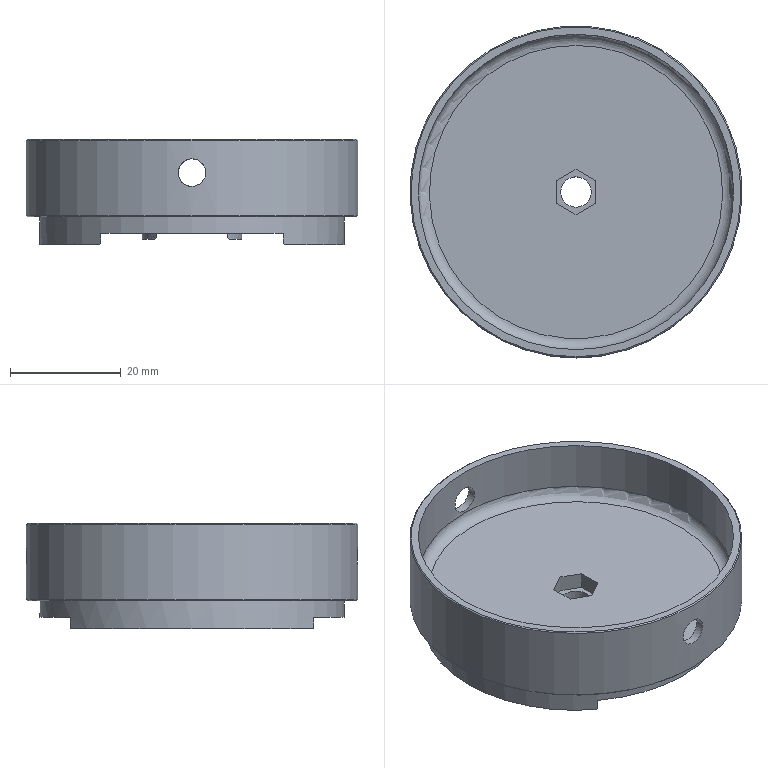NC program | NX | posted with a generic post | part box 60 x 60 x 19 mm
Lines 3548 to 4672 of 13134:
(ZLEVEL_PROFILE_COPY_COPY , TOOL : D10)
N7082 T09 M6
N7084 G54
N7086 G17 G0 G90 X8.096 Y19.918 S7500 M3
N7088 G43 Z30. H9
N7090 Z-7.5
N7092 G94 G1 Z-9. F1000.
N7094 X7.693 Y21.694
N7096 G3 X7.014 Y22.429 R1.
N7098 G1 X6.916 Y22.459 F850.
N7100 G3 X-6.888 Y22.468 R23.5
N7102 G1 X-6.895 Y22.435
N7104 X-6.91 Y22.461
N7106 G3 X7.014 Y22.429 R-23.5
N7108 X6.039 Y22.21 R1.
N7110 G1 X4.702 Y20.98
N7112 Z-7.5
N7114 G0 Z30.
(FLOOR_WALL_1_COPY_COPY , TOOL : D10)
N7116 X20.501 Y-0.848 S6500
N7118 Z-9.5
N7120 G1 Z-11. F1000.
N7122 G3 X21. Y0.018 R1.
N7124 G1 Y-0.017
N7126 G2 X16.334 Y-13.199 R21.
N7128 G1 X16.333 Y13.2
N7130 G3 X11.666 Y17.461 R21.
N7132 G1 X11.667 Y-17.461
N7134 G2 X7.001 Y-19.799 R21.
N7136 G1 X6.999 Y19.799
N7138 G3 X2.333 Y20.87 R21.
N7140 G1 X2.334 Y-20.87
N7142 G2 X-2.333 Y-20.87 R21.
N7144 G1 X-2.334 Y20.87
N7146 G3 X-7.001 Y19.799 R21.
N7148 G1 X-6.999 Y-19.799
N7150 G2 X-11.666 Y-17.461 R21.
N7152 G1 X-11.667 Y17.461
N7154 G3 X-16.334 Y13.199 R21.
N7156 G1 X-16.333 Y-13.2
N7158 G2 X-21. Y-0.018 R21.
N7160 G1 Y0.017
N7162 G2 X-20.5 Y0.883 R1.
N7164 G1 X-20.999
N7166 G3 X-21.5 Y0.017 R1.
N7168 G1 Y0.
N7170 G3 X0. Y-21.5 R21.5
N7172 X-21.5 Y0.017 R-21.5
N7174 X-21.001 Y-0.849 R1.
N7176 G1 X-19.947 Y-1.459
N7178 Z-9.5
N7180 G0 Z30.
N7182 M5
(ZLEVEL_PROFILE_COPY_1_COPY_COPY , TOOL : D6)
N7184 T07 M6
N7186 G54
N7188 G17 G0 G90 X22.978 Y11.057 S7500 M3
N7190 G43 Z30. H7
N7192 Z-7.45
N7194 G94 G1 X22.862 Y11.315 Z-7.465 F1000.
N7196 X22.193 Y12.577 Z-7.54
N7198 X21.131 Y14.29 Z-7.645
N7200 X19.937 Y15.913 Z-7.751
N7202 X18.619 Y17.437 Z-7.857
N7204 X17.185 Y18.852 Z-7.962
N7206 X15.643 Y20.15 Z-8.068
N7208 X14.004 Y21.322 Z-8.173
N7210 X12.277 Y22.361 Z-8.279
N7212 X10.474 Y23.26 Z-8.385
N7214 X8.605 Y24.014 Z-8.49
N7216 X6.683 Y24.618 Z-8.596
N7218 X4.719 Y25.069 Z-8.701
N7220 X2.725 Y25.363 Z-8.807
N7222 X0.715 Y25.499 Z-8.913
N7224 X0. Z-8.95
N7226 G3 X-25.499 Y0. R25.499 F2500.
N7228 X0. Y25.499 R-25.499
N7230 G1 X-0.168 Z-8.953
N7232 X-0.337 Y25.498 Z-8.956
N7234 X-0.505 Y25.492 Z-8.959
N7236 X-0.673 Y25.487 Z-8.962
N7238 X-0.842 Y25.482 Z-8.965
N7240 X-1.01 Y25.477 Z-8.968
N7242 X-1.179 Y25.472 Z-8.971
N7244 X-1.347 Y25.464 Z-8.974
N7246 X-1.515 Y25.454 Z-8.977
N7248 X-1.683 Y25.444 Z-8.98
N7250 X-1.851 Y25.431 Z-8.982
N7252 X-2.019 Y25.417 Z-8.985
N7254 X-2.187 Y25.403 Z-8.988
N7256 X-2.355 Y25.389 Z-8.991
N7258 X-2.523 Y25.375 Z-8.994
N7260 X-2.69 Y25.356 Z-8.997
N7262 X-2.858 Y25.339 Z-9.
N7264 X-3.025 Y25.32 Z-9.003
N7266 X-3.193 Y25.299 Z-9.006
N7268 X-3.36 Y25.278 Z-9.009
N7270 X-3.527 Y25.255 Z-9.012
N7272 X-3.693 Y25.231 Z-9.015
N7274 X-3.86 Y25.206 Z-9.018
N7276 X-4.027 Y25.18 Z-9.021
N7278 X-4.193 Y25.153 Z-9.024
N7280 X-4.359 Y25.124 Z-9.027
N7282 X-4.525 Y25.095 Z-9.03
N7284 X-4.691 Y25.065 Z-9.032
N7286 X-4.856 Y25.033 Z-9.035
N7288 X-5.021 Y25. Z-9.038
N7290 X-5.186 Y24.967 Z-9.041
N7292 X-5.351 Y24.932 Z-9.044
N7294 X-5.516 Y24.896 Z-9.047
N7296 X-5.68 Y24.859 Z-9.05
N7298 G3 X0. Y25.499 R-25.499
N7300 G1 X-0.168 Z-9.053
N7302 X-0.336 Y25.497 Z-9.056
N7304 X-0.504 Y25.494 Z-9.059
N7306 X-0.672 Y25.49 Z-9.062
N7308 X-0.841 Y25.485 Z-9.065
N7310 X-1.009 Y25.479 Z-9.068
N7312 X-1.177 Y25.472 Z-9.071
N7314 X-1.345 Y25.463 Z-9.074
N7316 X-1.513 Y25.454 Z-9.077
N7318 X-1.681 Y25.443 Z-9.079
N7320 X-1.849 Y25.431 Z-9.082
N7322 X-2.016 Y25.418 Z-9.085
N7324 X-2.184 Y25.404 Z-9.088
N7326 X-2.352 Y25.389 Z-9.091
N7328 X-2.519 Y25.373 Z-9.094
N7330 X-2.686 Y25.356 Z-9.097
N7332 X-2.854 Y25.337 Z-9.1
N7334 X-3.021 Y25.318 Z-9.103
N7336 X-3.188 Y25.297 Z-9.106
N7338 X-3.354 Y25.275 Z-9.109
N7340 X-3.521 Y25.253 Z-9.112
N7342 X-3.688 Y25.229 Z-9.115
N7344 X-3.854 Y25.204 Z-9.118
N7346 X-4.02 Y25.177 Z-9.121
N7348 X-4.186 Y25.15 Z-9.124
N7350 X-4.352 Y25.122 Z-9.126
N7352 X-4.518 Y25.092 Z-9.129
N7354 X-4.683 Y25.062 Z-9.132
N7356 X-4.848 Y25.03 Z-9.135
N7358 X-5.013 Y24.997 Z-9.138
N7360 X-5.178 Y24.964 Z-9.141
N7362 X-5.343 Y24.929 Z-9.144
N7364 X-5.507 Y24.893 Z-9.147
N7366 X-5.671 Y24.856 Z-9.15
N7368 G3 X0. Y25.494 R-25.494
N7370 G1 X-0.167 Z-9.153
N7372 X-0.335 Y25.492 Z-9.156
N7374 X-0.502 Y25.489 Z-9.159
N7376 X-0.67 Y25.485 Z-9.162
N7378 X-0.837 Y25.479 Z-9.165
N7380 X-1.005 Y25.473 Z-9.168
N7382 X-1.172 Y25.466 Z-9.17
N7384 X-1.34 Y25.457 Z-9.173
N7386 X-1.507 Y25.448 Z-9.176
N7388 X-1.674 Y25.437 Z-9.179
N7390 X-1.841 Y25.425 Z-9.182
N7392 X-2.008 Y25.412 Z-9.185
N7394 X-2.175 Y25.398 Z-9.188
N7396 X-2.342 Y25.383 Z-9.191
N7398 X-2.509 Y25.367 Z-9.194
N7400 X-2.676 Y25.349 Z-9.197
N7402 X-2.842 Y25.331 Z-9.2
N7404 X-3.009 Y25.312 Z-9.203
N7406 X-3.175 Y25.291 Z-9.206
N7408 X-3.341 Y25.269 Z-9.208
N7410 X-3.507 Y25.246 Z-9.211
N7412 X-3.673 Y25.222 Z-9.214
N7414 X-3.839 Y25.197 Z-9.217
N7416 X-4.004 Y25.171 Z-9.22
N7418 X-4.17 Y25.144 Z-9.223
N7420 X-4.335 Y25.116 Z-9.226
N7422 X-4.5 Y25.087 Z-9.229
N7424 X-4.664 Y25.056 Z-9.232
N7426 X-4.829 Y25.025 Z-9.235
N7428 X-4.993 Y24.992 Z-9.238
N7430 X-5.157 Y24.958 Z-9.241
N7432 X-5.321 Y24.923 Z-9.244
N7434 X-5.485 Y24.888 Z-9.247
N7436 X-5.648 Y24.851 Z-9.249
N7438 G3 X0. Y25.484 R-25.484
N7440 G1 X-0.166 Y25.483 Z-9.252
N7442 X-0.333 Y25.481 Z-9.255
N7444 X-0.499 Y25.478 Z-9.258
N7446 X-0.666 Y25.474 Z-9.261
N7448 X-0.832 Y25.469 Z-9.264
N7450 X-0.998 Y25.463 Z-9.267
N7452 X-1.165 Y25.455 Z-9.27
N7454 X-1.331 Y25.447 Z-9.273
N7456 X-1.497 Y25.437 Z-9.276
N7458 X-1.663 Y25.426 Z-9.279
N7460 X-1.829 Y25.414 Z-9.281
N7462 X-1.995 Y25.401 Z-9.284
N7464 X-2.161 Y25.387 Z-9.287
N7466 X-2.327 Y25.372 Z-9.29
N7468 X-2.493 Y25.356 Z-9.293
N7470 X-2.658 Y25.339 Z-9.296
N7472 X-2.824 Y25.321 Z-9.299
N7474 X-2.989 Y25.301 Z-9.302
N7476 X-3.154 Y25.281 Z-9.305
N7478 X-3.32 Y25.259 Z-9.308
N7480 X-3.484 Y25.236 Z-9.31
N7482 X-3.649 Y25.213 Z-9.313
N7484 X-3.814 Y25.188 Z-9.316
N7486 X-3.978 Y25.162 Z-9.319
N7488 X-4.142 Y25.135 Z-9.322
N7490 X-4.307 Y25.107 Z-9.325
N7492 X-4.47 Y25.078 Z-9.328
N7494 X-4.634 Y25.047 Z-9.331
N7496 X-4.798 Y25.016 Z-9.334
N7498 X-4.961 Y24.984 Z-9.337
N7500 X-5.124 Y24.95 Z-9.34
N7502 X-5.287 Y24.916 Z-9.342
N7504 X-5.449 Y24.88 Z-9.345
N7506 X-5.612 Y24.844 Z-9.348
N7508 G3 X0. Y25.469 R-25.469
N7510 G1 X-0.165 Y25.468 Z-9.351
N7512 X-0.33 Y25.466 Z-9.354
N7514 X-0.495 Y25.463 Z-9.357
N7516 X-0.66 Y25.459 Z-9.36
N7518 X-0.825 Y25.453 Z-9.363
N7520 X-0.989 Y25.447 Z-9.366
N7522 X-1.154 Y25.44 Z-9.368
N7524 X-1.319 Y25.431 Z-9.371
N7526 X-1.484 Y25.421 Z-9.374
N7528 X-1.648 Y25.411 Z-9.377
N7530 X-1.813 Y25.399 Z-9.38
N7532 X-1.978 Y25.386 Z-9.383
N7534 X-2.142 Y25.372 Z-9.386
N7536 X-2.306 Y25.357 Z-9.389
N7538 X-2.47 Y25.341 Z-9.391
N7540 X-2.635 Y25.324 Z-9.394
N7542 X-2.798 Y25.306 Z-9.397
N7544 X-2.962 Y25.287 Z-9.4
N7546 X-3.126 Y25.266 Z-9.403
N7548 X-3.29 Y25.245 Z-9.406
N7550 X-3.453 Y25.223 Z-9.409
N7552 X-3.616 Y25.199 Z-9.412
N7554 X-3.779 Y25.174 Z-9.415
N7556 X-3.942 Y25.149 Z-9.417
N7558 X-4.105 Y25.122 Z-9.42
N7560 X-4.268 Y25.094 Z-9.423
N7562 X-4.43 Y25.066 Z-9.426
N7564 X-4.592 Y25.036 Z-9.429
N7566 X-4.754 Y25.005 Z-9.432
N7568 X-4.916 Y24.973 Z-9.435
N7570 X-5.078 Y24.94 Z-9.438
N7572 X-5.239 Y24.906 Z-9.44
N7574 X-5.4 Y24.871 Z-9.443
N7576 X-5.561 Y24.835 Z-9.446
N7578 G3 X0. Y25.45 R-25.45
N7580 G1 X-0.163 Y25.448 Z-9.449
N7582 X-0.326 Y25.446 Z-9.452
N7584 X-0.489 Y25.443 Z-9.455
N7586 X-0.652 Y25.439 Z-9.458
N7588 X-0.815 Y25.433 Z-9.46
N7590 X-0.978 Y25.427 Z-9.463
N7592 X-1.141 Y25.419 Z-9.466
N7594 X-1.304 Y25.411 Z-9.469
N7596 X-1.467 Y25.401 Z-9.472
N7598 X-1.629 Y25.391 Z-9.475
N7600 X-1.792 Y25.379 Z-9.478
N7602 X-1.955 Y25.366 Z-9.48
N7604 X-2.117 Y25.352 Z-9.483
N7606 X-2.28 Y25.338 Z-9.486
N7608 X-2.442 Y25.322 Z-9.489
N7610 X-2.604 Y25.305 Z-9.492
N7612 X-2.766 Y25.287 Z-9.495
N7614 X-2.928 Y25.268 Z-9.497
N7616 X-3.09 Y25.248 Z-9.5
N7618 X-3.252 Y25.227 Z-9.503
N7620 X-3.413 Y25.205 Z-9.506
N7622 X-3.575 Y25.182 Z-9.509
N7624 X-3.736 Y25.158 Z-9.512
N7626 X-3.897 Y25.132 Z-9.515
N7628 X-4.058 Y25.106 Z-9.517
N7630 X-4.218 Y25.079 Z-9.52
N7632 X-4.379 Y25.051 Z-9.523
N7634 X-4.539 Y25.021 Z-9.526
N7636 X-4.7 Y24.991 Z-9.529
N7638 X-4.859 Y24.959 Z-9.532
N7640 X-5.019 Y24.927 Z-9.534
N7642 X-5.179 Y24.893 Z-9.537
N7644 X-5.338 Y24.859 Z-9.54
N7646 X-5.497 Y24.823 Z-9.543
N7648 G3 X0. Y25.425 R-25.425
N7650 G1 X-0.17 Y25.423 Z-9.546
N7652 X-0.341 Y25.421 Z-9.549
N7654 X-0.512 Y25.417 Z-9.552
N7656 X-0.683 Y25.412 Z-9.555
N7658 X-0.854 Y25.406 Z-9.558
N7660 X-1.024 Y25.399 Z-9.561
N7662 X-1.195 Y25.391 Z-9.564
N7664 X-1.366 Y25.381 Z-9.567
N7666 X-1.536 Y25.371 Z-9.57
N7668 X-1.707 Y25.359 Z-9.573
N7670 X-1.877 Y25.346 Z-9.576
N7672 X-2.047 Y25.332 Z-9.579
N7674 X-2.217 Y25.317 Z-9.582
N7676 X-2.387 Y25.3 Z-9.585
N7678 X-2.557 Y25.283 Z-9.588
N7680 X-2.727 Y25.264 Z-9.591
N7682 X-2.897 Y25.244 Z-9.594
N7684 X-3.066 Y25.223 Z-9.597
N7686 X-3.235 Y25.201 Z-9.6
N7688 X-3.405 Y25.178 Z-9.603
N7690 X-3.574 Y25.154 Z-9.606
N7692 X-3.742 Y25.128 Z-9.609
N7694 X-3.911 Y25.101 Z-9.612
N7696 X-4.079 Y25.074 Z-9.615
N7698 X-4.248 Y25.045 Z-9.618
N7700 X-4.416 Y25.015 Z-9.621
N7702 X-4.584 Y24.983 Z-9.624
N7704 X-4.751 Y24.951 Z-9.627
N7706 X-4.919 Y24.918 Z-9.63
N7708 X-5.086 Y24.883 Z-9.633
N7710 X-5.253 Y24.847 Z-9.635
N7712 X-5.419 Y24.81 Z-9.638
N7714 G3 X0. Y25.395 R-25.395
N7716 G1 X-0.168 Y25.394 Z-9.641
N7718 X-0.336 Y25.391 Z-9.644
N7720 X-0.503 Y25.387 Z-9.647
N7722 X-0.671 Y25.382 Z-9.65
N7724 X-0.839 Y25.376 Z-9.653
N7726 X-1.007 Y25.369 Z-9.656
N7728 X-1.175 Y25.361 Z-9.659
N7730 X-1.343 Y25.352 Z-9.662
N7732 X-1.51 Y25.341 Z-9.665
N7734 X-1.678 Y25.33 Z-9.668
N7736 X-1.845 Y25.317 Z-9.671
N7738 X-2.012 Y25.303 Z-9.674
N7740 X-2.18 Y25.288 Z-9.677
N7742 X-2.347 Y25.272 Z-9.68
N7744 X-2.514 Y25.255 Z-9.682
N7746 X-2.681 Y25.237 Z-9.685
N7748 X-2.848 Y25.218 Z-9.688
N7750 X-3.014 Y25.197 Z-9.691
N7752 X-3.181 Y25.176 Z-9.694
N7754 X-3.347 Y25.153 Z-9.697
N7756 X-3.513 Y25.129 Z-9.7
N7758 X-3.679 Y25.104 Z-9.703
N7760 X-3.845 Y25.078 Z-9.706
N7762 X-4.011 Y25.051 Z-9.709
N7764 X-4.176 Y25.023 Z-9.712
N7766 X-4.341 Y24.994 Z-9.715
N7768 X-4.506 Y24.963 Z-9.718
N7770 X-4.671 Y24.932 Z-9.721
N7772 X-4.836 Y24.899 Z-9.724
N7774 X-5. Y24.866 Z-9.726
N7776 X-5.164 Y24.831 Z-9.729
N7778 X-5.328 Y24.795 Z-9.732
N7780 G3 X0. Y25.361 R-25.361
N7782 G1 X-0.164 Y25.359 Z-9.735
N7784 X-0.329 Y25.357 Z-9.738
N7786 X-0.494 Y25.353 Z-9.741
N7788 X-0.658 Y25.348 Z-9.744
N7790 X-0.823 Y25.342 Z-9.747
N7792 X-0.987 Y25.335 Z-9.75
N7794 X-1.152 Y25.327 Z-9.752
N7796 X-1.316 Y25.318 Z-9.755
N7798 X-1.48 Y25.307 Z-9.758
N7800 X-1.645 Y25.296 Z-9.761
N7802 X-1.809 Y25.284 Z-9.764
N7804 X-1.973 Y25.27 Z-9.767
N7806 X-2.137 Y25.256 Z-9.77
N7808 X-2.301 Y25.24 Z-9.773
N7810 X-2.464 Y25.223 Z-9.775
N7812 X-2.628 Y25.206 Z-9.778
N7814 X-2.792 Y25.187 Z-9.781
N7816 X-2.955 Y25.167 Z-9.784
N7818 X-3.118 Y25.146 Z-9.787
N7820 X-3.281 Y25.124 Z-9.79
N7822 X-3.444 Y25.101 Z-9.793
N7824 X-3.607 Y25.077 Z-9.796
N7826 X-3.77 Y25.052 Z-9.798
N7828 X-3.932 Y25.025 Z-9.801
N7830 X-4.094 Y24.998 Z-9.804
N7832 X-4.256 Y24.97 Z-9.807
N7834 X-4.418 Y24.94 Z-9.81
N7836 X-4.58 Y24.91 Z-9.813
N7838 X-4.741 Y24.878 Z-9.816
N7840 X-4.902 Y24.846 Z-9.819
N7842 X-5.063 Y24.812 Z-9.821
N7844 X-5.224 Y24.777 Z-9.824
N7846 G3 X0. Y25.322 R-25.322
N7848 G1 X-0.171 Y25.32 Z-9.827
N7850 X-0.343 Y25.317 Z-9.83
N7852 X-0.515 Y25.313 Z-9.833
N7854 X-0.686 Y25.307 Z-9.836
N7856 X-0.858 Y25.301 Z-9.839
N7858 X-1.029 Y25.293 Z-9.842
N7860 X-1.201 Y25.284 Z-9.845
N7862 X-1.372 Y25.274 Z-9.848
N7864 X-1.543 Y25.263 Z-9.851
N7866 X-1.715 Y25.25 Z-9.854
N7868 X-1.886 Y25.237 Z-9.857
N7870 X-2.057 Y25.222 Z-9.86
N7872 X-2.227 Y25.206 Z-9.863
N7874 X-2.398 Y25.189 Z-9.866
N7876 X-2.569 Y25.17 Z-9.869
N7878 X-2.739 Y25.151 Z-9.872
N7880 X-2.91 Y25.13 Z-9.875
N7882 X-3.08 Y25.109 Z-9.878
N7884 X-3.25 Y25.086 Z-9.881
N7886 X-3.42 Y25.062 Z-9.884
N7888 X-3.589 Y25.036 Z-9.887
N7890 X-3.759 Y25.01 Z-9.89
N7892 X-3.928 Y24.983 Z-9.893
N7894 X-4.097 Y24.954 Z-9.896
N7896 X-4.266 Y24.924 Z-9.899
N7898 X-4.435 Y24.893 Z-9.902
N7900 X-4.603 Y24.861 Z-9.905
N7902 X-4.771 Y24.828 Z-9.908
N7904 X-4.939 Y24.793 Z-9.911
N7906 X-5.107 Y24.758 Z-9.914
N7908 G3 X0. Y25.279 R-25.279
N7910 G1 X-0.167 Y25.277 Z-9.917
N7912 X-0.334 Y25.274 Z-9.92
N7914 X-0.501 Y25.269 Z-9.923
N7916 X-0.669 Y25.264 Z-9.926
N7918 X-0.836 Y25.257 Z-9.929
N7920 X-1.003 Y25.25 Z-9.932
N7922 X-1.17 Y25.241 Z-9.935
N7924 X-1.337 Y25.231 Z-9.938
N7926 X-1.504 Y25.22 Z-9.941
N7928 X-1.671 Y25.208 Z-9.943
N7930 X-1.837 Y25.195 Z-9.946
N7932 X-2.004 Y25.181 Z-9.949
N7934 X-2.171 Y25.165 Z-9.952
N7936 X-2.337 Y25.149 Z-9.955
N7938 X-2.503 Y25.131 Z-9.958
N7940 X-2.669 Y25.113 Z-9.961
N7942 X-2.835 Y25.093 Z-9.964
N7944 X-3.001 Y25.072 Z-9.967
N7946 X-3.167 Y25.05 Z-9.97
N7948 X-3.332 Y25.027 Z-9.973
N7950 X-3.498 Y25.002 Z-9.976
N7952 X-3.663 Y24.977 Z-9.978
N7954 X-3.828 Y24.951 Z-9.981
N7956 X-3.993 Y24.923 Z-9.984
N7958 X-4.157 Y24.895 Z-9.987
N7960 X-4.322 Y24.865 Z-9.99
N7962 X-4.486 Y24.834 Z-9.993
N7964 X-4.65 Y24.802 Z-9.996
N7966 X-4.814 Y24.769 Z-9.999
N7968 X-4.977 Y24.735 Z-10.002
N7970 G3 X0. Y25.231 R-25.231
N7972 G1 X-0.162 Y25.229 Z-10.005
N7974 X-0.325 Y25.226 Z-10.008
N7976 X-0.487 Y25.221 Z-10.01
N7978 X-0.649 Y25.216 Z-10.013
N7980 X-0.812 Y25.21 Z-10.016
N7982 X-0.974 Y25.202 Z-10.019
N7984 X-1.136 Y25.194 Z-10.022
N7986 X-1.299 Y25.184 Z-10.025
N7988 X-1.461 Y25.174 Z-10.027
N7990 X-1.623 Y25.162 Z-10.03
N7992 X-1.785 Y25.149 Z-10.033
N7994 X-1.946 Y25.136 Z-10.036
N7996 X-2.108 Y25.121 Z-10.039
N7998 X-2.27 Y25.105 Z-10.042
N8000 X-2.431 Y25.088 Z-10.044
N8002 X-2.593 Y25.07 Z-10.047
N8004 X-2.754 Y25.051 Z-10.05
N8006 X-2.915 Y25.031 Z-10.053
N8008 X-3.076 Y25.01 Z-10.056
N8010 X-3.237 Y24.988 Z-10.059
N8012 X-3.397 Y24.965 Z-10.061
N8014 X-3.558 Y24.941 Z-10.064
N8016 X-3.718 Y24.916 Z-10.067
N8018 X-3.878 Y24.889 Z-10.07
N8020 X-4.038 Y24.862 Z-10.073
N8022 X-4.198 Y24.834 Z-10.076
N8024 X-4.358 Y24.804 Z-10.078
N8026 X-4.517 Y24.774 Z-10.081
N8028 X-4.676 Y24.743 Z-10.084
N8030 X-4.835 Y24.71 Z-10.087
N8032 G3 X0. Y25.179 R-25.179
N8034 G1 X-0.168 Y25.176 Z-10.09
N8036 X-0.337 Y25.173 Z-10.093
N8038 X-0.505 Y25.168 Z-10.096
N8040 X-0.674 Y25.162 Z-10.099
N8042 X-0.842 Y25.155 Z-10.102
N8044 X-1.01 Y25.147 Z-10.105
N8046 X-1.178 Y25.138 Z-10.108
N8048 X-1.347 Y25.127 Z-10.111
N8050 X-1.515 Y25.116 Z-10.113
N8052 X-1.683 Y25.103 Z-10.116
N8054 X-1.85 Y25.089 Z-10.119
N8056 X-2.018 Y25.074 Z-10.122
N8058 X-2.186 Y25.058 Z-10.125
N8060 X-2.353 Y25.041 Z-10.128
N8062 X-2.521 Y25.023 Z-10.131
N8064 X-2.688 Y25.003 Z-10.134
N8066 X-2.855 Y24.983 Z-10.137
N8068 X-3.022 Y24.961 Z-10.14
N8070 X-3.189 Y24.938 Z-10.143
N8072 X-3.355 Y24.914 Z-10.146
N8074 X-3.522 Y24.889 Z-10.149
N8076 X-3.688 Y24.863 Z-10.152
N8078 X-3.854 Y24.836 Z-10.155
N8080 X-4.02 Y24.807 Z-10.158
N8082 X-4.186 Y24.778 Z-10.161
N8084 X-4.351 Y24.747 Z-10.163
N8086 X-4.516 Y24.715 Z-10.166
N8088 X-4.681 Y24.683 Z-10.169
N8090 G3 X0. Y25.123 R-25.123
N8092 G1 X-0.162 Y25.12 Z-10.172
N8094 X-0.325 Y25.116 Z-10.175
N8096 X-0.487 Y25.112 Z-10.178
N8098 X-0.649 Y25.106 Z-10.181
N8100 X-0.812 Y25.099 Z-10.184
N8102 X-0.974 Y25.091 Z-10.186
N8104 X-1.136 Y25.082 Z-10.189
N8106 X-1.299 Y25.072 Z-10.192
N8108 X-1.461 Y25.061 Z-10.195
N8110 X-1.623 Y25.049 Z-10.198
N8112 X-1.784 Y25.036 Z-10.201
N8114 X-1.946 Y25.022 Z-10.203
N8116 X-2.108 Y25.007 Z-10.206
N8118 X-2.269 Y24.99 Z-10.209
N8120 X-2.431 Y24.973 Z-10.212
N8122 X-2.592 Y24.955 Z-10.215
N8124 X-2.753 Y24.935 Z-10.218
N8126 X-2.914 Y24.915 Z-10.22
N8128 X-3.075 Y24.893 Z-10.223
N8130 X-3.236 Y24.87 Z-10.226
N8132 X-3.397 Y24.847 Z-10.229
N8134 X-3.557 Y24.822 Z-10.232
N8136 X-3.717 Y24.796 Z-10.235
N8138 X-3.877 Y24.77 Z-10.237
N8140 X-4.037 Y24.742 Z-10.24
N8142 X-4.197 Y24.713 Z-10.243
N8144 X-4.356 Y24.683 Z-10.246
N8146 X-4.515 Y24.652 Z-10.249
N8148 G3 X0. Y25.062 R-25.062
N8150 G1 X-0.168 Y25.059 Z-10.252
N8152 X-0.336 Y25.055 Z-10.255
N8154 X-0.504 Y25.05 Z-10.258
N8156 X-0.672 Y25.044 Z-10.261
N8158 X-0.84 Y25.036 Z-10.263
N8160 X-1.008 Y25.028 Z-10.266
N8162 X-1.175 Y25.018 Z-10.269
N8164 X-1.343 Y25.007 Z-10.272
N8166 X-1.511 Y24.995 Z-10.275
N8168 X-1.678 Y24.982 Z-10.278
N8170 X-1.845 Y24.968 Z-10.281
N8172 X-2.013 Y24.952 Z-10.284
N8174 X-2.18 Y24.936 Z-10.287
N8176 X-2.347 Y24.918 Z-10.29
N8178 X-2.514 Y24.899 Z-10.293
N8180 X-2.68 Y24.88 Z-10.296
N8182 X-2.847 Y24.858 Z-10.299
N8184 X-3.013 Y24.836 Z-10.302
N8186 X-3.18 Y24.813 Z-10.305
N8188 X-3.346 Y24.789 Z-10.307
N8190 X-3.512 Y24.763 Z-10.31
N8192 X-3.677 Y24.737 Z-10.313
N8194 X-3.843 Y24.709 Z-10.316
N8196 X-4.008 Y24.68 Z-10.319
N8198 X-4.173 Y24.65 Z-10.322
N8200 X-4.338 Y24.619 Z-10.325
N8202 G3 X0. Y24.998 R-24.998
N8204 G1 X-0.16 Y24.995 Z-10.328
N8206 X-0.321 Y24.991 Z-10.331
N8208 X-0.482 Y24.986 Z-10.334
N8210 X-0.643 Y24.98 Z-10.336
N8212 X-0.803 Y24.973 Z-10.339
N8214 X-0.964 Y24.964 Z-10.342
N8216 X-1.124 Y24.955 Z-10.345
N8218 X-1.285 Y24.945 Z-10.348
N8220 X-1.445 Y24.933 Z-10.35
N8222 X-1.605 Y24.921 Z-10.353
N8224 X-1.765 Y24.908 Z-10.356
N8226 X-1.925 Y24.893 Z-10.359
N8228 X-2.085 Y24.878 Z-10.362
N8230 X-2.245 Y24.861 Z-10.364
N8232 X-2.405 Y24.844 Z-10.367
N8234 X-2.564 Y24.825 Z-10.37
N8236 X-2.723 Y24.805 Z-10.373
N8238 X-2.883 Y24.785 Z-10.376
N8240 X-3.042 Y24.763 Z-10.378
N8242 X-3.201 Y24.74 Z-10.381
N8244 X-3.359 Y24.716 Z-10.384
N8246 X-3.518 Y24.692 Z-10.387
N8248 X-3.676 Y24.666 Z-10.39
N8250 X-3.835 Y24.639 Z-10.392
N8252 X-3.993 Y24.611 Z-10.395
N8254 X-4.15 Y24.582 Z-10.398
N8256 G3 X0. Y24.93 R-24.93
N8258 G1 X-0.165 Y24.927 Z-10.401
N8260 X-0.331 Y24.922 Z-10.404
N8262 X-0.497 Y24.917 Z-10.407
N8264 X-0.663 Y24.91 Z-10.41
N8266 X-0.828 Y24.902 Z-10.413
N8268 X-0.994 Y24.893 Z-10.415
N8270 X-1.159 Y24.883 Z-10.418
N8272 X-1.325 Y24.872 Z-10.421
N8274 X-1.49 Y24.86 Z-10.424
N8276 X-1.655 Y24.846 Z-10.427
N8278 X-1.82 Y24.832 Z-10.43
N8280 X-1.985 Y24.816 Z-10.433
N8282 X-2.15 Y24.799 Z-10.436
N8284 X-2.314 Y24.782 Z-10.439
N8286 X-2.479 Y24.763 Z-10.442
N8288 X-2.643 Y24.743 Z-10.444
N8290 X-2.807 Y24.721 Z-10.447
N8292 X-2.971 Y24.699 Z-10.45
N8294 X-3.135 Y24.676 Z-10.453
N8296 X-3.299 Y24.651 Z-10.456
N8298 X-3.462 Y24.626 Z-10.459
N8300 X-3.626 Y24.599 Z-10.462
N8302 X-3.789 Y24.571 Z-10.465
N8304 X-3.952 Y24.543 Z-10.468
N8306 G3 X0. Y24.859 R-24.859
N8308 G1 X-0.171 Y24.855 Z-10.471
N8310 X-0.342 Y24.85 Z-10.474
N8312 X-0.513 Y24.844 Z-10.477
N8314 X-0.684 Y24.836 Z-10.48
N8316 X-0.856 Y24.828 Z-10.483
N8318 X-1.027 Y24.818 Z-10.486
N8320 X-1.197 Y24.807 Z-10.489
N8322 X-1.368 Y24.795 Z-10.491
N8324 X-1.539 Y24.781 Z-10.494
N8326 X-1.709 Y24.767 Z-10.497
N8328 X-1.88 Y24.751 Z-10.5
N8330 X-2.05 Y24.734 Z-10.503
N8332 X-2.22 Y24.716 Z-10.506
N8334 X-2.39 Y24.697 Z-10.509
N8336 X-2.56 Y24.676 Z-10.512
N8338 X-2.73 Y24.655 Z-10.515
N8340 X-2.899 Y24.632 Z-10.518
N8342 X-3.068 Y24.608 Z-10.521
N8344 X-3.237 Y24.582 Z-10.524
N8346 X-3.406 Y24.556 Z-10.527
N8348 X-3.575 Y24.528 Z-10.53
N8350 X-3.743 Y24.5 Z-10.533
N8352 G3 X0. Y24.784 R-24.784
N8354 G1 X-0.161 Y24.78 Z-10.536
N8356 X-0.322 Y24.775 Z-10.539
N8358 X-0.483 Y24.769 Z-10.542
N8360 X-0.644 Y24.762 Z-10.545
N8362 X-0.805 Y24.754 Z-10.547
N8364 X-0.966 Y24.745 Z-10.55
N8366 X-1.127 Y24.734 Z-10.553
N8368 X-1.288 Y24.723 Z-10.556
N8370 X-1.449 Y24.711 Z-10.559
N8372 X-1.609 Y24.697 Z-10.562
N8374 X-1.77 Y24.683 Z-10.564
N8376 X-1.93 Y24.667 Z-10.567
N8378 X-2.09 Y24.651 Z-10.57
N8380 X-2.251 Y24.633 Z-10.573
N8382 X-2.411 Y24.614 Z-10.576
N8384 X-2.57 Y24.594 Z-10.578
N8386 X-2.73 Y24.573 Z-10.581
N8388 X-2.889 Y24.552 Z-10.584
N8390 X-3.049 Y24.529 Z-10.587
N8392 X-3.208 Y24.505 Z-10.59
N8394 X-3.367 Y24.48 Z-10.592
N8396 X-3.526 Y24.453 Z-10.595
N8398 G3 X0. Y24.706 R-24.706
N8400 G1 X-0.166 Y24.702 Z-10.598
N8402 X-0.331 Y24.696 Z-10.601
N8404 X-0.497 Y24.69 Z-10.604
N8406 X-0.663 Y24.682 Z-10.607
N8408 X-0.829 Y24.673 Z-10.61
N8410 X-0.994 Y24.663 Z-10.613
N8412 X-1.16 Y24.652 Z-10.616
N8414 X-1.325 Y24.639 Z-10.618
N8416 X-1.491 Y24.626 Z-10.621
N8418 X-1.656 Y24.611 Z-10.624
N8420 X-1.821 Y24.596 Z-10.627
N8422 X-1.986 Y24.579 Z-10.63
N8424 X-2.15 Y24.561 Z-10.633
N8426 X-2.315 Y24.542 Z-10.636
N8428 X-2.479 Y24.521 Z-10.639
N8430 X-2.644 Y24.5 Z-10.642
N8432 X-2.808 Y24.478 Z-10.645
N8434 X-2.972 Y24.454 Z-10.647
N8436 X-3.135 Y24.429 Z-10.65
N8438 X-3.299 Y24.404 Z-10.653
N8440 G3 X0. Y24.625 R-24.625
N8442 G1 X-0.171 Y24.62 Z-10.656
N8444 X-0.342 Y24.614 Z-10.659
N8446 X-0.513 Y24.607 Z-10.662
N8448 X-0.684 Y24.598 Z-10.665
N8450 X-0.855 Y24.588 Z-10.668
N8452 X-1.026 Y24.577 Z-10.671
N8454 X-1.196 Y24.565 Z-10.674
N8456 X-1.367 Y24.552 Z-10.677
N8458 X-1.537 Y24.537 Z-10.68
N8460 X-1.708 Y24.521 Z-10.683
N8462 X-1.878 Y24.504 Z-10.686
N8464 X-2.048 Y24.485 Z-10.689
N8466 X-2.218 Y24.466 Z-10.692
N8468 X-2.387 Y24.445 Z-10.695
N8470 X-2.557 Y24.423 Z-10.698
N8472 X-2.726 Y24.4 Z-10.701
N8474 X-2.895 Y24.376 Z-10.704
N8476 X-3.064 Y24.35 Z-10.707
N8478 G3 X0. Y24.542 R-24.542
N8480 G1 X-0.157 Y24.537 Z-10.71
N8482 X-0.315 Y24.531 Z-10.713
N8484 X-0.472 Y24.524 Z-10.715
N8486 X-0.63 Y24.516 Z-10.718
N8488 X-0.787 Y24.507 Z-10.721
N8490 X-0.944 Y24.496 Z-10.724
N8492 X-1.101 Y24.485 Z-10.726
N8494 X-1.258 Y24.473 Z-10.729
N8496 X-1.415 Y24.459 Z-10.732
N8498 X-1.572 Y24.445 Z-10.735
N8500 X-1.728 Y24.43 Z-10.737
N8502 X-1.885 Y24.413 Z-10.74
N8504 X-2.041 Y24.396 Z-10.743
N8506 X-2.197 Y24.377 Z-10.746
N8508 X-2.354 Y24.358 Z-10.748
N8510 X-2.509 Y24.337 Z-10.751
N8512 X-2.665 Y24.316 Z-10.754
N8514 X-2.821 Y24.293 Z-10.757
N8516 G3 X0. Y24.456 R-24.456
N8518 G1 X-0.161 Y24.45 Z-10.759
N8520 X-0.323 Y24.444 Z-10.762
N8522 X-0.484 Y24.436 Z-10.765
N8524 X-0.645 Y24.427 Z-10.768
N8526 X-0.807 Y24.417 Z-10.771
N8528 X-0.968 Y24.405 Z-10.774
N8530 X-1.129 Y24.393 Z-10.776
N8532 X-1.29 Y24.379 Z-10.779
N8534 X-1.45 Y24.365 Z-10.782
N8536 X-1.611 Y24.349 Z-10.785
N8538 X-1.771 Y24.332 Z-10.788
N8540 X-1.932 Y24.315 Z-10.79
N8542 X-2.092 Y24.296 Z-10.793
N8544 X-2.252 Y24.276 Z-10.796
N8546 X-2.411 Y24.254 Z-10.799
N8548 X-2.571 Y24.232 Z-10.802
N8550 G3 X0. Y24.368 R-24.368
N8552 G1 X-0.166 Y24.362 Z-10.805
N8554 X-0.332 Y24.354 Z-10.808
N8556 X-0.498 Y24.345 Z-10.81
N8558 X-0.663 Y24.335 Z-10.813
N8560 X-0.829 Y24.323 Z-10.816
N8562 X-0.995 Y24.311 Z-10.819
N8564 X-1.16 Y24.297 Z-10.822
N8566 X-1.325 Y24.282 Z-10.825
N8568 X-1.491 Y24.266 Z-10.828
N8570 X-1.656 Y24.249 Z-10.831
N8572 X-1.82 Y24.23 Z-10.834
N8574 X-1.985 Y24.211 Z-10.837
N8576 X-2.149 Y24.19 Z-10.839
N8578 X-2.314 Y24.168 Z-10.842
N8580 G3 X0. Y24.278 R-24.278
N8582 G1 X-0.171 Y24.271 Z-10.845
N8584 X-0.343 Y24.262 Z-10.848
N8586 X-0.515 Y24.251 Z-10.851
N8588 X-0.686 Y24.24 Z-10.854
N8590 X-0.857 Y24.227 Z-10.857
N8592 X-1.029 Y24.212 Z-10.86
N8594 X-1.199 Y24.197 Z-10.863
N8596 X-1.37 Y24.18 Z-10.866
N8598 X-1.541 Y24.162 Z-10.869
N8600 X-1.711 Y24.143 Z-10.872
N8602 X-1.882 Y24.122 Z-10.875
N8604 X-2.052 Y24.1 Z-10.878
N8606 G3 X0. Y24.187 R-24.187
N8608 G1 X-0.149 Y24.179 Z-10.881
N8610 X-0.298 Y24.171 Z-10.884
N8612 X-0.448 Y24.161 Z-10.886
N8614 X-0.597 Y24.15 Z-10.889
N8616 X-0.746 Y24.139 Z-10.891
N8618 X-0.895 Y24.126 Z-10.894
N8620 X-1.043 Y24.112 Z-10.897
N8622 X-1.192 Y24.097 Z-10.899
N8624 X-1.34 Y24.082 Z-10.902
N8626 X-1.489 Y24.065 Z-10.904
N8628 X-1.637 Y24.047 Z-10.907
N8630 X-1.785 Y24.028 Z-10.91
N8632 G3 X0. Y24.094 R-24.094
N8634 G1 X-0.151 Y24.085 Z-10.912
N8636 X-0.302 Y24.075 Z-10.915
N8638 X-0.453 Y24.064 Z-10.918
N8640 X-0.604 Y24.052 Z-10.92
N8642 X-0.755 Y24.038 Z-10.923
N8644 X-0.906 Y24.024 Z-10.925
N8646 X-1.056 Y24.008 Z-10.928
N8648 X-1.206 Y23.991 Z-10.931
N8650 X-1.357 Y23.973 Z-10.933
N8652 X-1.507 Y23.954 Z-10.936
N8654 G3 X0. Y24.002 R-24.002
N8656 G1 X-0.155 Y23.991 Z-10.939
N8658 X-0.309 Y23.978 Z-10.941
N8660 X-0.464 Y23.965 Z-10.944
N8662 X-0.619 Y23.95 Z-10.947
N8664 X-0.773 Y23.934 Z-10.95
N8666 X-0.927 Y23.916 Z-10.952
N8668 X-1.081 Y23.897 Z-10.955
N8670 X-1.235 Y23.877 Z-10.958
N8672 G3 X0. Y23.909 R-23.909
N8674 G1 X-0.158 Y23.895 Z-10.96
N8676 X-0.316 Y23.88 Z-10.963
N8678 X-0.474 Y23.862 Z-10.966
N8680 X-0.632 Y23.844 Z-10.969
N8682 X-0.789 Y23.823 Z-10.972
N8684 X-0.946 Y23.801 Z-10.974
N8686 G3 X0. Y23.819 R-23.819
N8688 G1 X-0.166 Y23.8 Z-10.977
N8690 X-0.333 Y23.779 Z-10.98
N8692 X-0.499 Y23.755 Z-10.983
N8694 X-0.664 Y23.727 Z-10.986
N8696 G3 X0. Y23.737 R-23.737
N8698 G1 X-0.133 Y23.716 Z-10.988
N8700 X-0.267 Y23.692 Z-10.991
N8702 X-0.4 Y23.664 Z-10.993
N8704 X-0.533 Y23.631 Z-10.995
N8706 X-0.599 Y23.611 Z-10.996
N8708 X-0.666 Y23.587 Z-10.998
N8710 X-0.732 Y23.589 Z-10.999
N8712 X-0.799 Y23.586 Z-11.
N8714 G3 X-23.586 Y-0.799 R23.6
N8716 X-0.799 Y23.586 R-23.6
N8718 G1 Z-9.6
N8720 G0 Z30.
N8722 M5
(ZLEVEL_PROFILE_COPY_1_COPY_COPY_COPY , TOOL : D4)
N8724 T22 M6
N8726 G54
N8728 G17 G0 G90 X-0.498 Y-1.55 S5000 M3
N8730 G43 Z30. H22
N8732 Z-9.6
N8734 G94 G1 X0.895 Z-9.673 F1000.
N8736 X1.79 Y0. Z-9.767
N8738 X0.895 Y1.55 Z-9.861
N8740 X-0.895 Z-9.954
N8742 X-1.79 Y0. Z-10.048
N8744 X-0.895 Y-1.55 Z-10.142
N8746 X0.895 Z-10.236
N8748 X1.79 Y0. Z-10.33
N8750 X0.895 Y1.55 Z-10.423
N8752 X-0.895 Z-10.517
N8754 X-1.79 Y0. Z-10.611
N8756 X-0.895 Y-1.55 Z-10.705
N8758 X0.895 Z-10.799
N8760 X1.79 Y0. Z-10.892
N8762 X0.895 Y1.55 Z-10.986
N8764 X-0.895 Z-11.08
N8766 X-1.79 Y0. F1650.
N8768 X-0.895 Y-1.55
N8770 X0.895
N8772 X1.79 Y0.
N8774 X0.895 Y1.55
N8776 X-0.895
N8778 X-1.79 Y0. Z-11.111
N8780 X-0.895 Y-1.55 Z-11.142
N8782 X0.109 Z-11.16
N8784 X0.895
N8786 X1.79 Y0.
N8788 X0.895 Y1.55
N8790 X-0.895
N8792 X-1.79 Y0. Z-11.191
N8794 X-0.895 Y-1.55 Z-11.222
N8796 X0.109 Z-11.24
N8798 X0.895
N8800 X1.79 Y0.
N8802 X0.895 Y1.55
N8804 X-0.895
N8806 X-1.79 Y0. Z-11.271
N8808 X-0.895 Y-1.55 Z-11.302
N8810 X0.109 Z-11.32
N8812 X0.895
N8814 X1.79 Y0.
N8816 X0.895 Y1.55
N8818 X-0.895
N8820 X-1.79 Y0. Z-11.351
N8822 X-0.895 Y-1.55 Z-11.382
N8824 X0.109 Z-11.4
N8826 X0.895
N8828 X1.79 Y0.
N8830 X0.895 Y1.55
N8832 X-0.895
N8834 X-1.79 Y0. Z-11.431
N8836 X-0.895 Y-1.55 Z-11.462
N8838 X0.109 Z-11.48
N8840 X0.895
N8842 X1.79 Y0.
N8844 X0.895 Y1.55
N8846 X-0.895
N8848 X-1.79 Y0. Z-11.511
N8850 X-0.895 Y-1.55 Z-11.542
N8852 X0.109 Z-11.56
N8854 X0.895
N8856 X1.79 Y0.
N8858 X0.895 Y1.55
N8860 X-0.895
N8862 X-1.79 Y0. Z-11.591
N8864 X-0.895 Y-1.55 Z-11.622
N8866 X0.109 Z-11.64
N8868 X0.895
N8870 X1.79 Y0.
N8872 X0.895 Y1.55
N8874 X-0.895
N8876 X-1.79 Y0. Z-11.671
N8878 X-0.895 Y-1.55 Z-11.702
N8880 X0.109 Z-11.72
N8882 X0.895
N8884 X1.79 Y0.
N8886 X0.895 Y1.55
N8888 X-0.895
N8890 X-1.79 Y0. Z-11.751
N8892 X-0.895 Y-1.55 Z-11.782
N8894 X0.109 Z-11.8
N8896 X0.895
N8898 X1.79 Y0.
N8900 X0.895 Y1.55
N8902 X-0.895
N8904 X-1.79 Y0. Z-11.831
N8906 X-0.895 Y-1.55 Z-11.862
N8908 X0.109 Z-11.88
N8910 X0.895
N8912 X1.79 Y0.
N8914 X0.895 Y1.55
N8916 X-0.895
N8918 X-1.79 Y0. Z-11.911
N8920 X-0.895 Y-1.55 Z-11.942
N8922 X0.109 Z-11.96
N8924 X0.895
N8926 X1.79 Y0.
N8928 X0.895 Y1.55
N8930 X-0.895
N8932 X-1.79 Y0. Z-11.991
N8934 X-0.895 Y-1.55 Z-12.022
N8936 X0.109 Z-12.04
N8938 X0.895
N8940 X1.79 Y0.
N8942 X0.895 Y1.55
N8944 X-0.895
N8946 X-1.79 Y0. Z-12.071
N8948 X-0.895 Y-1.55 Z-12.102
N8950 X0.109 Z-12.12
N8952 X0.895
N8954 X1.79 Y0.
N8956 X0.895 Y1.55
N8958 X-0.895
N8960 X-1.79 Y0. Z-12.151
N8962 X-0.895 Y-1.55 Z-12.182
N8964 X0.109 Z-12.2
N8966 X0.895
N8968 X1.79 Y0.
N8970 X0.895 Y1.55
N8972 X-0.895
N8974 X-1.79 Y0. Z-12.231
N8976 X-0.895 Y-1.55 Z-12.262
N8978 X0.109 Z-12.28
N8980 X0.895
N8982 X1.79 Y0.
N8984 X0.895 Y1.55
N8986 X-0.895
N8988 X-1.79 Y0. Z-12.311
N8990 X-0.895 Y-1.55 Z-12.342
N8992 X0.109 Z-12.36
N8994 X0.895
N8996 X1.79 Y0.
N8998 X0.895 Y1.55
N9000 X-0.895
N9002 X-1.79 Y0. Z-12.391
N9004 X-0.895 Y-1.55 Z-12.422
N9006 X0.109 Z-12.44
N9008 X0.895
N9010 X1.79 Y0.
N9012 X0.895 Y1.55
N9014 X-0.895
N9016 X-1.79 Y0. Z-12.471
N9018 X-0.895 Y-1.55 Z-12.502
N9020 X0.109 Z-12.52
N9022 X0.895
N9024 X1.79 Y0.
N9026 X0.895 Y1.55
N9028 X-0.895
N9030 X-1.79 Y0. Z-12.551
N9032 X-0.895 Y-1.55 Z-12.582
N9034 X0.109 Z-12.6
N9036 X0.895
N9038 X1.79 Y0.
N9040 X0.895 Y1.55
N9042 X-0.895
N9044 X-1.79 Y0. Z-12.631
N9046 X-0.895 Y-1.55 Z-12.662
N9048 X0.109 Z-12.68
N9050 X0.895
N9052 X1.79 Y0.
N9054 X0.895 Y1.55
N9056 X-0.895
N9058 X-1.79 Y0. Z-12.711
N9060 X-0.895 Y-1.55 Z-12.742
N9062 X0.109 Z-12.76
N9064 X0.895
N9066 X1.79 Y0.
N9068 X0.895 Y1.55
N9070 X-0.895
N9072 X-1.79 Y0. Z-12.791
N9074 X-0.895 Y-1.55 Z-12.822
N9076 X0.109 Z-12.84
N9078 X0.895
N9080 X1.79 Y0.
N9082 X0.895 Y1.55
N9084 X-0.895
N9086 X-1.79 Y0. Z-12.871
N9088 X-0.895 Y-1.55 Z-12.902
N9090 X0.109 Z-12.92
N9092 X0.895
N9094 X1.79 Y0.
N9096 X0.895 Y1.55
N9098 X-0.895
N9100 X-1.79 Y0. Z-12.951
N9102 X-0.895 Y-1.55 Z-12.982
N9104 X0.109 Z-13.
N9106 X0.895
N9108 X1.79 Y0.
N9110 X0.895 Y1.55
N9112 X-0.895
N9114 X-1.79 Y0. Z-13.031
N9116 X-0.895 Y-1.55 Z-13.062
N9118 X0.109 Z-13.08
N9120 X0.895
N9122 X1.79 Y0.
N9124 X0.895 Y1.55
N9126 X-0.895
N9128 X-1.79 Y0. Z-13.111
N9130 X-0.895 Y-1.55 Z-13.142
N9132 X0.109 Z-13.16
N9134 X0.895
N9136 X1.79 Y0.
N9138 X0.895 Y1.55
N9140 X-0.895
N9142 X-1.79 Y0. Z-13.191
N9144 X-0.895 Y-1.55 Z-13.222
N9146 X0.109 Z-13.24
N9148 X0.895
N9150 X1.79 Y0.
N9152 X0.895 Y1.55
N9154 X-0.895
N9156 X-1.79 Y0. Z-13.271
N9158 X-0.895 Y-1.55 Z-13.302
N9160 X0.109 Z-13.32
N9162 X0.895
N9164 X1.79 Y0.
N9166 X0.895 Y1.55
N9168 X-0.895
N9170 X-1.79 Y0. Z-13.351
N9172 X-0.895 Y-1.55 Z-13.382
N9174 X0.109 Z-13.4
N9176 X0.895
N9178 X1.79 Y0.
N9180 X0.895 Y1.55
N9182 X-0.895
N9184 X-1.79 Y0. Z-13.431
N9186 X-0.895 Y-1.55 Z-13.462
N9188 X0.109 Z-13.48
N9190 X0.895
N9192 X1.79 Y0.
N9194 X0.895 Y1.55
N9196 X-0.895
N9198 X-1.79 Y0. Z-13.511
N9200 X-0.895 Y-1.55 Z-13.542
N9202 X0.109 Z-13.56
N9204 X0.895
N9206 X1.79 Y0.
N9208 X0.895 Y1.55
N9210 X-0.895
N9212 X-1.79 Y0. Z-13.591
N9214 X-0.895 Y-1.55 Z-13.622
N9216 X0.109 Z-13.64
N9218 X0.895
N9220 X1.79 Y0.
N9222 X0.895 Y1.55
N9224 X-0.895
N9226 X-1.79 Y0. Z-13.671
N9228 X-0.895 Y-1.55 Z-13.702
N9230 X0.109 Z-13.72
N9232 X0.895
N9234 X1.79 Y0.
N9236 X0.895 Y1.55
N9238 X-0.895
N9240 X-1.79 Y0. Z-13.751
N9242 X-0.895 Y-1.55 Z-13.782
N9244 X-0.464 Z-13.79
N9246 X0.895
N9248 X1.79 Y0.
N9250 X0.895 Y1.55
N9252 X-0.895
N9254 X-1.79 Y0. Z-13.821
N9256 X-0.895 Y-1.55 Z-13.852
N9258 X-0.464 Z-13.86
N9260 X0.895
N9262 X1.79 Y0.
N9264 X0.895 Y1.55
N9266 X-0.895
N9268 X-1.79 Y0. Z-13.891
N9270 X-0.895 Y-1.55 Z-13.922
N9272 X-0.464 Z-13.93
N9274 X0.895
N9276 X1.79 Y0.
N9278 X0.895 Y1.55
N9280 X-0.895
N9282 X-1.79 Y0. Z-13.961
N9284 X-0.895 Y-1.55 Z-13.992
N9286 X-0.464 Z-14.
N9288 X0.895
N9290 X1.79 Y0.
N9292 X0.895 Y1.55
N9294 X-0.895
N9296 X-1.79 Y0.
N9298 X-0.895 Y-1.55
N9300 X-0.464
N9302 Z-12.6
N9304 G0 Z30.
N9306 M5